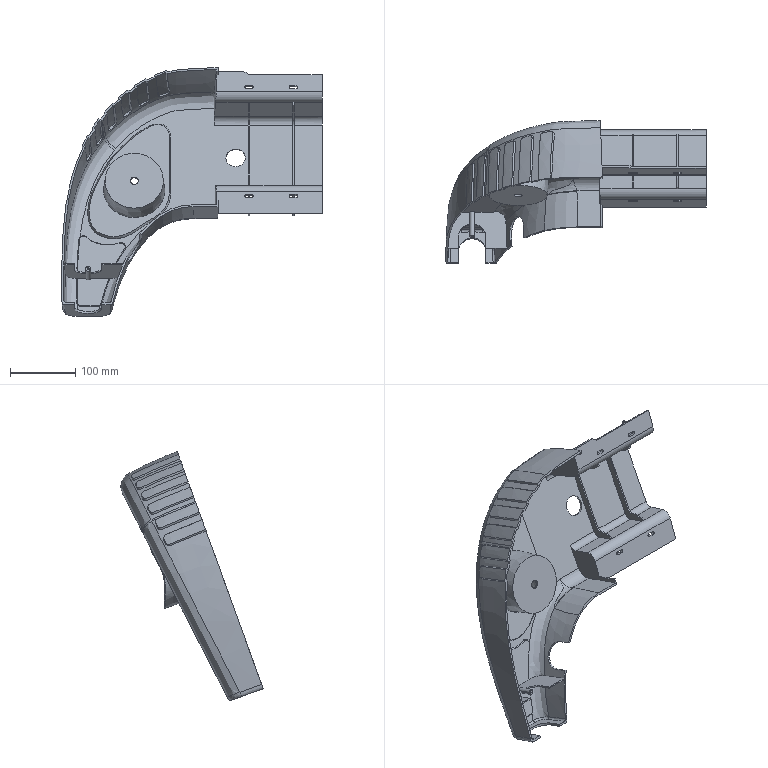Part | STEP file | Consen Cover R | 1 solid | 463 faces | box 398.708 x 218.09 x 381.338 mm | volume 568981 mm3 | plane 216 | spline 156 | cylinder 89 | cone 2 | commonest cylinder face diameters 4.623 x17 4.657 x13 20 x12 5 x8 9 x8 16 x4